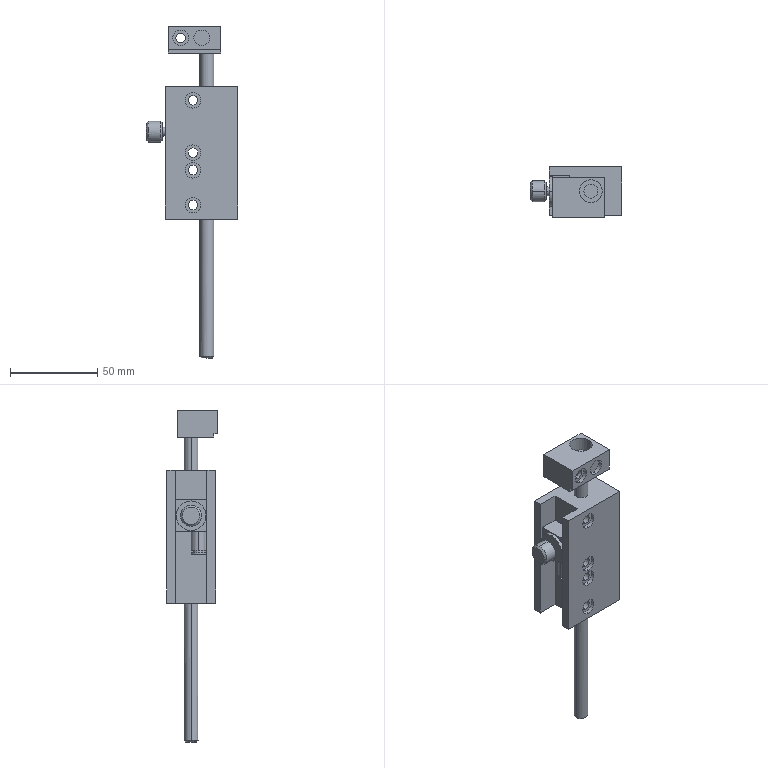Part | STEP file | 00193112_FESTSTELLEINH._BKP-HMPL-12-80.100 | 1 solid | 105 faces | box 52.1 x 29 x 190 mm | volume 85928 mm3 | cylinder 54 | plane 43 | cone 8 | commonest cylinder face diameters 9 x20 5.5 x10 8 x10 4 x2 5 x2 6 x2